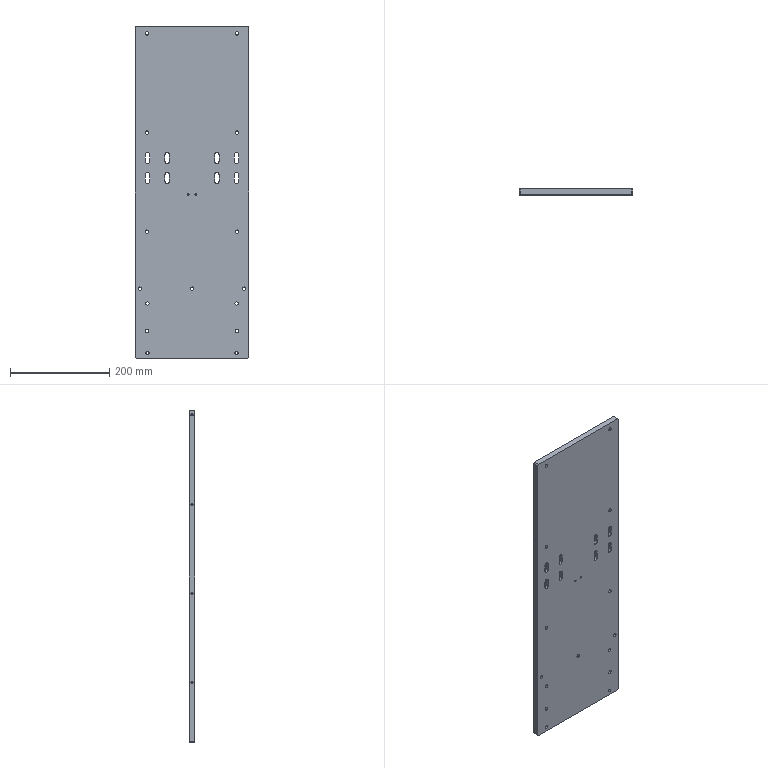Part | SolidWorks | features HoleWzd 6, Chamfer 1, Extrusion 1, MirrorPattern 1 | 1 solid | 185 faces | box 230 x 12 x 670 mm | volume 1812577 mm3 | cylinder 112 | plane 57 | cone 16 | commonest cylinder face diameters 9 x24 15 x24 4.2 x16 6.8 x16 6.6 x14 11 x14